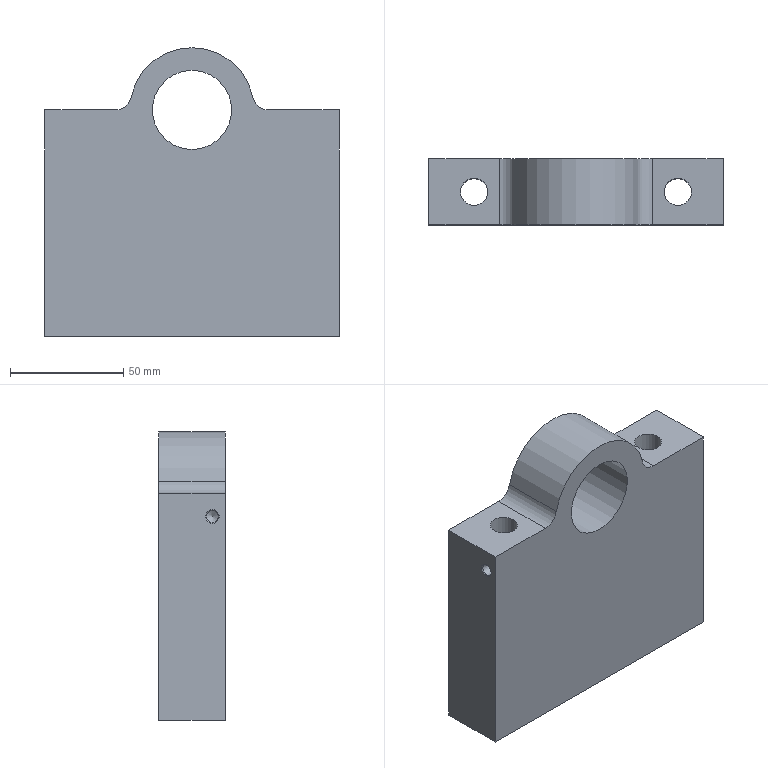Part | STEP file | YBQDJ-PD-7 | 1 solid | 22 faces | box 130 x 29.2 x 127.5 mm | volume 362195 mm3 | cylinder 9 | plane 7 | cone 6 | commonest cylinder face diameters 5.2 x2 12 x2 14 x2 8.5 x1 35 x1 55 x1